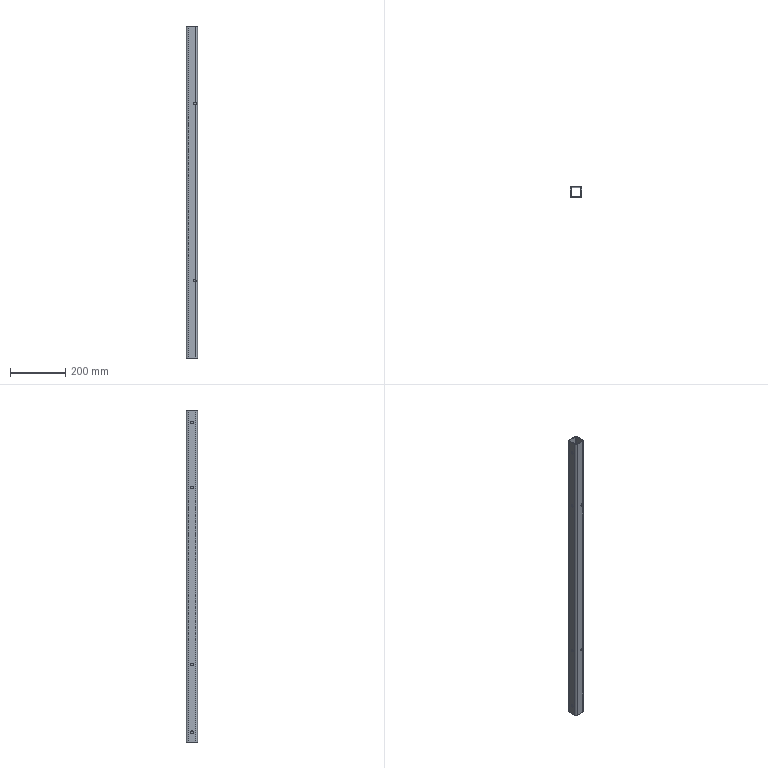Part | STEP file | DIN 59 410 - 40x40x2.9-1000_ZD_01 | 1 solid | 24 faces | box 40 x 40 x 1200 mm | volume 489076 mm3 | cylinder 14 | plane 10 | commonest cylinder face diameters 10 x6 5.8 x4 11.6 x4